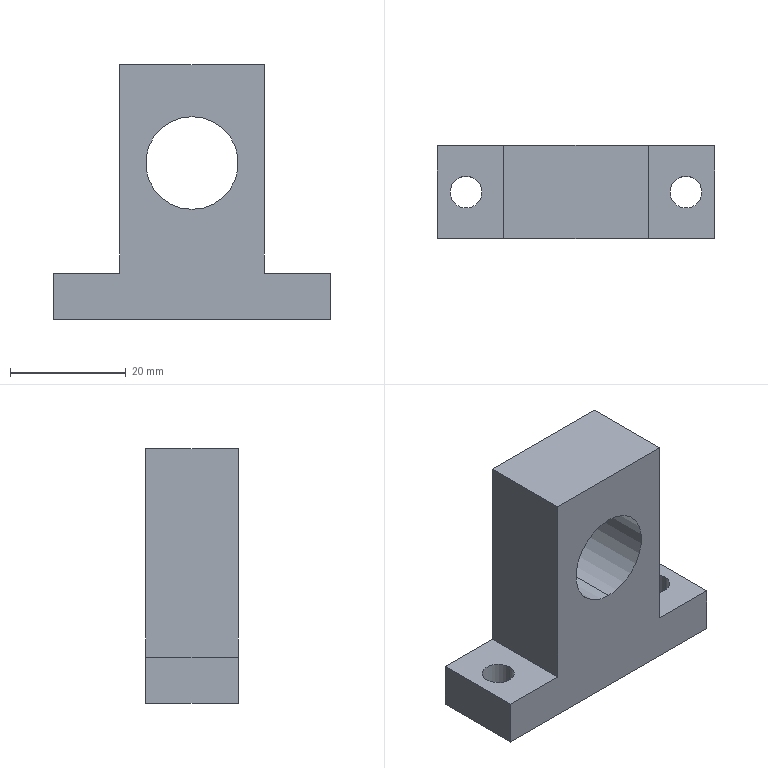Part | SolidWorks | features BaseBody 1 | 1 solid | 16 faces | box 48 x 16 x 44 mm | volume 16947 mm3 | plane 10 | cylinder 6 | commonest cylinder face diameters 5.5 x4 16 x2
STEP:
#1=CARTESIAN_POINT('',(0.,8.,19.));
#2=VERTEX_POINT('',#1);
#3=CARTESIAN_POINT('',(0.,8.,35.));
#4=VERTEX_POINT('',#3);
#5=CARTESIAN_POINT('',(0.,8.,27.));
#6=DIRECTION('',(0.,1.,0.));
#7=DIRECTION('',(0.,0.,-1.));
#8=AXIS2_PLACEMENT_3D('',#5,#6,#7);
#9=CIRCLE('',#8,8.);
#10=EDGE_CURVE('',#2,#4,#9,.T.);
#11=ORIENTED_EDGE('',*,*,#10,.T.);
#12=CARTESIAN_POINT('',(0.,-8.,35.));
#13=VERTEX_POINT('',#12);
#14=CARTESIAN_POINT('',(0.,8.,35.));
#15=DIRECTION('',(0.,-1.,0.));
#16=VECTOR('',#15,1000.);
#17=LINE('',#14,#16);
#18=EDGE_CURVE('',#4,#13,#17,.T.);
#19=ORIENTED_EDGE('',*,*,#18,.T.);
#20=CARTESIAN_POINT('',(0.,-8.,19.));
#21=VERTEX_POINT('',#20);
#22=CARTESIAN_POINT('',(0.,-8.,27.));
#23=DIRECTION('',(0.,1.,0.));
#24=DIRECTION('',(0.,0.,-1.));
#25=AXIS2_PLACEMENT_3D('',#22,#23,#24);
#26=CIRCLE('',#25,8.);
#27=EDGE_CURVE('',#21,#13,#26,.T.);
#28=ORIENTED_EDGE('',*,*,#27,.F.);
#29=CARTESIAN_POINT('',(0.,8.,19.));
#30=DIRECTION('',(0.,-1.,0.));
#31=VECTOR('',#30,1000.);
#32=LINE('',#29,#31);
#33=EDGE_CURVE('',#2,#21,#32,.T.);
#34=ORIENTED_EDGE('',*,*,#33,.F.);
#35=EDGE_LOOP('',(#11,#19,#28,#34));
#36=FACE_OUTER_BOUND('',#35,.T.);
#37=CARTESIAN_POINT('',(0.,8.,27.));
#38=DIRECTION('',(0.,-1.,0.));
#39=DIRECTION('',(0.,0.,-1.));
#40=AXIS2_PLACEMENT_3D('',#37,#38,#39);
#41=CYLINDRICAL_SURFACE('',#40,8.);
#42=ADVANCED_FACE('',(#36),#41,.F.);
#43=CARTESIAN_POINT('',(16.25,0.,8.));
#44=VERTEX_POINT('',#43);
#45=CARTESIAN_POINT('',(21.75,0.,8.));
#46=VERTEX_POINT('',#45);
#47=CARTESIAN_POINT('',(19.,0.,8.));
#48=DIRECTION('',(0.,0.,1.));
#49=DIRECTION('',(-1.,0.,0.));
#50=AXIS2_PLACEMENT_3D('',#47,#48,#49);
#51=CIRCLE('',#50,2.75);
#52=EDGE_CURVE('',#44,#46,#51,.T.);
#53=ORIENTED_EDGE('',*,*,#52,.T.);
#54=CARTESIAN_POINT('',(21.75,0.,0.));
#55=VERTEX_POINT('',#54);
#56=CARTESIAN_POINT('',(21.75,0.,8.));
#57=DIRECTION('',(0.,0.,-1.));
#58=VECTOR('',#57,1000.);
#59=LINE('',#56,#58);
#60=EDGE_CURVE('',#46,#55,#59,.T.);
#61=ORIENTED_EDGE('',*,*,#60,.T.);
#62=CARTESIAN_POINT('',(16.25,0.,0.));
#63=VERTEX_POINT('',#62);
#64=CARTESIAN_POINT('',(19.,0.,0.));
#65=DIRECTION('',(0.,0.,1.));
#66=DIRECTION('',(-1.,0.,0.));
#67=AXIS2_PLACEMENT_3D('',#64,#65,#66);
#68=CIRCLE('',#67,2.75);
#69=EDGE_CURVE('',#63,#55,#68,.T.);
#70=ORIENTED_EDGE('',*,*,#69,.F.);
#71=CARTESIAN_POINT('',(16.25,0.,8.));
#72=DIRECTION('',(0.,0.,-1.));
#73=VECTOR('',#72,1000.);
#74=LINE('',#71,#73);
#75=EDGE_CURVE('',#44,#63,#74,.T.);
#76=ORIENTED_EDGE('',*,*,#75,.F.);
#77=EDGE_LOOP('',(#53,#61,#70,#76));
#78=FACE_OUTER_BOUND('',#77,.T.);
#79=CARTESIAN_POINT('',(19.,0.,8.));
#80=DIRECTION('',(0.,0.,-1.));
#81=DIRECTION('',(-1.,0.,0.));
#82=AXIS2_PLACEMENT_3D('',#79,#80,#81);
#83=CYLINDRICAL_SURFACE('',#82,2.75);
#84=ADVANCED_FACE('',(#78),#83,.F.);
#85=CARTESIAN_POINT('',(-21.75,0.,8.));
#86=VERTEX_POINT('',#85);
#87=CARTESIAN_POINT('',(-16.25,0.,8.));
#88=VERTEX_POINT('',#87);
#89=CARTESIAN_POINT('',(-19.,0.,8.));
#90=DIRECTION('',(0.,0.,1.));
#91=DIRECTION('',(-1.,0.,0.));
#92=AXIS2_PLACEMENT_3D('',#89,#90,#91);
#93=CIRCLE('',#92,2.75);
#94=EDGE_CURVE('',#86,#88,#93,.T.);
#95=ORIENTED_EDGE('',*,*,#94,.T.);
#96=CARTESIAN_POINT('',(-16.25,0.,0.));
#97=VERTEX_POINT('',#96);
#98=CARTESIAN_POINT('',(-16.25,0.,8.));
#99=DIRECTION('',(0.,0.,-1.));
#100=VECTOR('',#99,1000.);
#101=LINE('',#98,#100);
#102=EDGE_CURVE('',#88,#97,#101,.T.);
#103=ORIENTED_EDGE('',*,*,#102,.T.);
#104=CARTESIAN_POINT('',(-21.75,0.,0.));
#105=VERTEX_POINT('',#104);
#106=CARTESIAN_POINT('',(-19.,0.,0.));
#107=DIRECTION('',(0.,0.,1.));
#108=DIRECTION('',(-1.,0.,0.));
#109=AXIS2_PLACEMENT_3D('',#106,#107,#108);
#110=CIRCLE('',#109,2.75);
#111=EDGE_CURVE('',#105,#97,#110,.T.);
#112=ORIENTED_EDGE('',*,*,#111,.F.);
#113=CARTESIAN_POINT('',(-21.75,0.,8.));
#114=DIRECTION('',(0.,0.,-1.));
#115=VECTOR('',#114,1000.);
#116=LINE('',#113,#115);
#117=EDGE_CURVE('',#86,#105,#116,.T.);
#118=ORIENTED_EDGE('',*,*,#117,.F.);
#119=EDGE_LOOP('',(#95,#103,#112,#118));
#120=FACE_OUTER_BOUND('',#119,.T.);
#121=CARTESIAN_POINT('',(-19.,0.,8.));
#122=DIRECTION('',(0.,0.,-1.));
#123=DIRECTION('',(-1.,0.,0.));
#124=AXIS2_PLACEMENT_3D('',#121,#122,#123);
#125=CYLINDRICAL_SURFACE('',#124,2.75);
#126=ADVANCED_FACE('',(#120),#125,.F.);
#127=ORIENTED_EDGE('',*,*,#10,.F.);
#128=CARTESIAN_POINT('',(0.,8.,27.));
#129=DIRECTION('',(0.,1.,0.));
#130=DIRECTION('',(0.,0.,-1.));
#131=AXIS2_PLACEMENT_3D('',#128,#129,#130);
#132=CIRCLE('',#131,8.);
#133=EDGE_CURVE('',#4,#2,#132,.T.);
#134=ORIENTED_EDGE('',*,*,#133,.F.);
#135=EDGE_LOOP('',(#127,#134));
#136=FACE_BOUND('',#135,.T.);
#137=CARTESIAN_POINT('',(-24.,8.,8.));
#138=VERTEX_POINT('',#137);
#139=CARTESIAN_POINT('',(-24.,8.,0.));
#140=VERTEX_POINT('',#139);
#141=CARTESIAN_POINT('',(-24.,8.,8.));
#142=DIRECTION('',(0.,0.,-1.));
#143=VECTOR('',#142,1000.);
#144=LINE('',#141,#143);
#145=EDGE_CURVE('',#138,#140,#144,.T.);
#146=ORIENTED_EDGE('',*,*,#145,.F.);
#147=CARTESIAN_POINT('',(-12.5,8.,8.));
#148=VERTEX_POINT('',#147);
#149=CARTESIAN_POINT('',(-24.,8.,8.));
#150=DIRECTION('',(-1.,0.,0.));
#151=VECTOR('',#150,1000.);
#152=LINE('',#149,#151);
#153=EDGE_CURVE('',#148,#138,#152,.T.);
#154=ORIENTED_EDGE('',*,*,#153,.F.);
#155=CARTESIAN_POINT('',(-12.5,8.,44.));
#156=VERTEX_POINT('',#155);
#157=CARTESIAN_POINT('',(-12.5,8.,8.));
#158=DIRECTION('',(0.,0.,-1.));
#159=VECTOR('',#158,1000.);
#160=LINE('',#157,#159);
#161=EDGE_CURVE('',#156,#148,#160,.T.);
#162=ORIENTED_EDGE('',*,*,#161,.F.);
#163=CARTESIAN_POINT('',(12.5,8.,44.));
#164=VERTEX_POINT('',#163);
#165=CARTESIAN_POINT('',(-24.,8.,44.));
#166=DIRECTION('',(-1.,0.,0.));
#167=VECTOR('',#166,1000.);
#168=LINE('',#165,#167);
#169=EDGE_CURVE('',#164,#156,#168,.T.);
#170=ORIENTED_EDGE('',*,*,#169,.F.);
#171=CARTESIAN_POINT('',(12.5,8.,8.));
#172=VERTEX_POINT('',#171);
#173=CARTESIAN_POINT('',(12.5,8.,8.));
#174=DIRECTION('',(0.,0.,1.));
#175=VECTOR('',#174,1000.);
#176=LINE('',#173,#175);
#177=EDGE_CURVE('',#172,#164,#176,.T.);
#178=ORIENTED_EDGE('',*,*,#177,.F.);
#179=CARTESIAN_POINT('',(24.,8.,8.));
#180=VERTEX_POINT('',#179);
#181=CARTESIAN_POINT('',(-24.,8.,8.));
#182=DIRECTION('',(-1.,0.,0.));
#183=VECTOR('',#182,1000.);
#184=LINE('',#181,#183);
#185=EDGE_CURVE('',#180,#172,#184,.T.);
#186=ORIENTED_EDGE('',*,*,#185,.F.);
#187=CARTESIAN_POINT('',(24.,8.,0.));
#188=VERTEX_POINT('',#187);
#189=CARTESIAN_POINT('',(24.,8.,8.));
#190=DIRECTION('',(0.,0.,1.));
#191=VECTOR('',#190,1000.);
#192=LINE('',#189,#191);
#193=EDGE_CURVE('',#188,#180,#192,.T.);
#194=ORIENTED_EDGE('',*,*,#193,.F.);
#195=CARTESIAN_POINT('',(-24.,8.,0.));
#196=DIRECTION('',(1.,0.,0.));
#197=VECTOR('',#196,1000.);
#198=LINE('',#195,#197);
#199=EDGE_CURVE('',#140,#188,#198,.T.);
#200=ORIENTED_EDGE('',*,*,#199,.F.);
#201=EDGE_LOOP('',(#146,#154,#162,#170,#178,#186,#194,#200));
#202=FACE_OUTER_BOUND('',#201,.T.);
#203=CARTESIAN_POINT('',(-24.,8.,8.));
#204=DIRECTION('',(0.,-1.,0.));
#205=DIRECTION('',(0.,0.,-1.));
#206=AXIS2_PLACEMENT_3D('',#203,#204,#205);
#207=PLANE('',#206);
#208=ADVANCED_FACE('',(#136,#202),#207,.F.);
#209=ORIENTED_EDGE('',*,*,#18,.F.);
#210=ORIENTED_EDGE('',*,*,#133,.T.);
#211=ORIENTED_EDGE('',*,*,#33,.T.);
#212=CARTESIAN_POINT('',(0.,-8.,27.));
#213=DIRECTION('',(0.,1.,0.));
#214=DIRECTION('',(0.,0.,-1.));
#215=AXIS2_PLACEMENT_3D('',#212,#213,#214);
#216=CIRCLE('',#215,8.);
#217=EDGE_CURVE('',#13,#21,#216,.T.);
#218=ORIENTED_EDGE('',*,*,#217,.F.);
#219=EDGE_LOOP('',(#209,#210,#211,#218));
#220=FACE_OUTER_BOUND('',#219,.T.);
#221=CARTESIAN_POINT('',(0.,8.,27.));
#222=DIRECTION('',(0.,-1.,0.));
#223=DIRECTION('',(0.,0.,-1.));
#224=AXIS2_PLACEMENT_3D('',#221,#222,#223);
#225=CYLINDRICAL_SURFACE('',#224,8.);
#226=ADVANCED_FACE('',(#220),#225,.F.);
#227=ORIENTED_EDGE('',*,*,#69,.T.);
#228=CARTESIAN_POINT('',(19.,0.,0.));
#229=DIRECTION('',(0.,0.,1.));
#230=DIRECTION('',(-1.,0.,0.));
#231=AXIS2_PLACEMENT_3D('',#228,#229,#230);
#232=CIRCLE('',#231,2.75);
#233=EDGE_CURVE('',#55,#63,#232,.T.);
#234=ORIENTED_EDGE('',*,*,#233,.T.);
#235=EDGE_LOOP('',(#227,#234));
#236=FACE_BOUND('',#235,.T.);
#237=CARTESIAN_POINT('',(-24.,-8.,0.));
#238=VERTEX_POINT('',#237);
#239=CARTESIAN_POINT('',(-24.,0.,0.));
#240=DIRECTION('',(0.,1.,0.));
#241=VECTOR('',#240,1000.);
#242=LINE('',#239,#241);
#243=EDGE_CURVE('',#238,#140,#242,.T.);
#244=ORIENTED_EDGE('',*,*,#243,.T.);
#245=ORIENTED_EDGE('',*,*,#199,.T.);
#246=CARTESIAN_POINT('',(24.,-8.,0.));
#247=VERTEX_POINT('',#246);
#248=CARTESIAN_POINT('',(24.,0.,0.));
#249=DIRECTION('',(0.,-1.,0.));
#250=VECTOR('',#249,1000.);
#251=LINE('',#248,#250);
#252=EDGE_CURVE('',#188,#247,#251,.T.);
#253=ORIENTED_EDGE('',*,*,#252,.T.);
#254=CARTESIAN_POINT('',(0.,-8.,0.));
#255=DIRECTION('',(-1.,0.,0.));
#256=VECTOR('',#255,1000.);
#257=LINE('',#254,#256);
#258=EDGE_CURVE('',#247,#238,#257,.T.);
#259=ORIENTED_EDGE('',*,*,#258,.T.);
#260=EDGE_LOOP('',(#244,#245,#253,#259));
#261=FACE_OUTER_BOUND('',#260,.T.);
#262=ORIENTED_EDGE('',*,*,#111,.T.);
#263=CARTESIAN_POINT('',(-19.,0.,0.));
#264=DIRECTION('',(0.,0.,1.));
#265=DIRECTION('',(-1.,0.,0.));
#266=AXIS2_PLACEMENT_3D('',#263,#264,#265);
#267=CIRCLE('',#266,2.75);
#268=EDGE_CURVE('',#97,#105,#267,.T.);
#269=ORIENTED_EDGE('',*,*,#268,.T.);
#270=EDGE_LOOP('',(#262,#269));
#271=FACE_BOUND('',#270,.T.);
#272=CARTESIAN_POINT('',(0.,0.,0.));
#273=DIRECTION('',(0.,0.,-1.));
#274=DIRECTION('',(-1.,0.,0.));
#275=AXIS2_PLACEMENT_3D('',#272,#273,#274);
#276=PLANE('',#275);
#277=ADVANCED_FACE('',(#236,#261,#271),#276,.T.);
#278=CARTESIAN_POINT('',(-24.,-8.,8.));
#279=VERTEX_POINT('',#278);
#280=CARTESIAN_POINT('',(-24.,-8.,8.));
#281=DIRECTION('',(0.,0.,-1.));
#282=VECTOR('',#281,1000.);
#283=LINE('',#280,#282);
#284=EDGE_CURVE('',#279,#238,#283,.T.);
#285=ORIENTED_EDGE('',*,*,#284,.F.);
#286=CARTESIAN_POINT('',(-24.,-8.,8.));
#287=DIRECTION('',(0.,-1.,0.));
#288=VECTOR('',#287,1000.);
#289=LINE('',#286,#288);
#290=EDGE_CURVE('',#138,#279,#289,.T.);
#291=ORIENTED_EDGE('',*,*,#290,.F.);
#292=ORIENTED_EDGE('',*,*,#145,.T.);
#293=ORIENTED_EDGE('',*,*,#243,.F.);
#294=EDGE_LOOP('',(#285,#291,#292,#293));
#295=FACE_OUTER_BOUND('',#294,.T.);
#296=CARTESIAN_POINT('',(-24.,-8.,8.));
#297=DIRECTION('',(1.,0.,0.));
#298=DIRECTION('',(0.,0.,-1.));
#299=AXIS2_PLACEMENT_3D('',#296,#297,#298);
#300=PLANE('',#299);
#301=ADVANCED_FACE('',(#295),#300,.F.);
#302=ORIENTED_EDGE('',*,*,#153,.T.);
#303=ORIENTED_EDGE('',*,*,#290,.T.);
#304=CARTESIAN_POINT('',(-12.5,-8.,8.));
#305=VERTEX_POINT('',#304);
#306=CARTESIAN_POINT('',(0.,-8.,8.));
#307=DIRECTION('',(-1.,0.,0.));
#308=VECTOR('',#307,1000.);
#309=LINE('',#306,#308);
#310=EDGE_CURVE('',#305,#279,#309,.T.);
#311=ORIENTED_EDGE('',*,*,#310,.F.);
#312=CARTESIAN_POINT('',(-12.5,0.,8.));
#313=DIRECTION('',(0.,-1.,0.));
#314=VECTOR('',#313,1000.);
#315=LINE('',#312,#314);
#316=EDGE_CURVE('',#148,#305,#315,.T.);
#317=ORIENTED_EDGE('',*,*,#316,.F.);
#318=EDGE_LOOP('',(#302,#303,#311,#317));
#319=FACE_OUTER_BOUND('',#318,.T.);
#320=ORIENTED_EDGE('',*,*,#94,.F.);
#321=CARTESIAN_POINT('',(-19.,0.,8.));
#322=DIRECTION('',(0.,0.,1.));
#323=DIRECTION('',(-1.,0.,0.));
#324=AXIS2_PLACEMENT_3D('',#321,#322,#323);
#325=CIRCLE('',#324,2.75);
#326=EDGE_CURVE('',#88,#86,#325,.T.);
#327=ORIENTED_EDGE('',*,*,#326,.F.);
#328=EDGE_LOOP('',(#320,#327));
#329=FACE_BOUND('',#328,.T.);
#330=CARTESIAN_POINT('',(0.,0.,8.));
#331=DIRECTION('',(0.,0.,-1.));
#332=DIRECTION('',(-1.,0.,0.));
#333=AXIS2_PLACEMENT_3D('',#330,#331,#332);
#334=PLANE('',#333);
#335=ADVANCED_FACE('',(#319,#329),#334,.F.);
#336=ORIENTED_EDGE('',*,*,#161,.T.);
#337=ORIENTED_EDGE('',*,*,#316,.T.);
#338=CARTESIAN_POINT('',(-12.5,-8.,44.));
#339=VERTEX_POINT('',#338);
#340=CARTESIAN_POINT('',(-12.5,-8.,8.));
#341=DIRECTION('',(0.,0.,1.));
#342=VECTOR('',#341,1000.);
#343=LINE('',#340,#342);
#344=EDGE_CURVE('',#305,#339,#343,.T.);
#345=ORIENTED_EDGE('',*,*,#344,.T.);
#346=CARTESIAN_POINT('',(-12.5,8.,44.));
#347=DIRECTION('',(0.,1.,0.));
#348=VECTOR('',#347,1000.);
#349=LINE('',#346,#348);
#350=EDGE_CURVE('',#339,#156,#349,.T.);
#351=ORIENTED_EDGE('',*,*,#350,.T.);
#352=EDGE_LOOP('',(#336,#337,#345,#351));
#353=FACE_OUTER_BOUND('',#352,.T.);
#354=CARTESIAN_POINT('',(-12.5,8.,8.));
#355=DIRECTION('',(-1.,0.,0.));
#356=DIRECTION('',(0.,0.,1.));
#357=AXIS2_PLACEMENT_3D('',#354,#355,#356);
#358=PLANE('',#357);
#359=ADVANCED_FACE('',(#353),#358,.T.);
#360=ORIENTED_EDGE('',*,*,#169,.T.);
#361=ORIENTED_EDGE('',*,*,#350,.F.);
#362=CARTESIAN_POINT('',(12.5,-8.,44.));
#363=VERTEX_POINT('',#362);
#364=CARTESIAN_POINT('',(-12.5,-8.,44.));
#365=DIRECTION('',(1.,0.,0.));
#366=VECTOR('',#365,1000.);
#367=LINE('',#364,#366);
#368=EDGE_CURVE('',#339,#363,#367,.T.);
#369=ORIENTED_EDGE('',*,*,#368,.T.);
#370=CARTESIAN_POINT('',(12.5,8.,44.));
#371=DIRECTION('',(0.,1.,0.));
#372=VECTOR('',#371,1000.);
#373=LINE('',#370,#372);
#374=EDGE_CURVE('',#363,#164,#373,.T.);
#375=ORIENTED_EDGE('',*,*,#374,.T.);
#376=EDGE_LOOP('',(#360,#361,#369,#375));
#377=FACE_OUTER_BOUND('',#376,.T.);
#378=CARTESIAN_POINT('',(-12.5,8.,44.));
#379=DIRECTION('',(0.,0.,1.));
#380=DIRECTION('',(1.,0.,0.));
#381=AXIS2_PLACEMENT_3D('',#378,#379,#380);
#382=PLANE('',#381);
#383=ADVANCED_FACE('',(#377),#382,.T.);
#384=ORIENTED_EDGE('',*,*,#177,.T.);
#385=ORIENTED_EDGE('',*,*,#374,.F.);
#386=CARTESIAN_POINT('',(12.5,-8.,8.));
#387=VERTEX_POINT('',#386);
#388=CARTESIAN_POINT('',(12.5,-8.,44.));
#389=DIRECTION('',(0.,0.,-1.));
#390=VECTOR('',#389,1000.);
#391=LINE('',#388,#390);
#392=EDGE_CURVE('',#363,#387,#391,.T.);
#393=ORIENTED_EDGE('',*,*,#392,.T.);
#394=CARTESIAN_POINT('',(12.5,8.,8.));
#395=DIRECTION('',(0.,1.,0.));
#396=VECTOR('',#395,1000.);
#397=LINE('',#394,#396);
#398=EDGE_CURVE('',#387,#172,#397,.T.);
#399=ORIENTED_EDGE('',*,*,#398,.T.);
#400=EDGE_LOOP('',(#384,#385,#393,#399));
#401=FACE_OUTER_BOUND('',#400,.T.);
#402=CARTESIAN_POINT('',(12.5,8.,44.));
#403=DIRECTION('',(1.,0.,0.));
#404=DIRECTION('',(0.,0.,-1.));
#405=AXIS2_PLACEMENT_3D('',#402,#403,#404);
#406=PLANE('',#405);
#407=ADVANCED_FACE('',(#401),#406,.T.);
#408=ORIENTED_EDGE('',*,*,#52,.F.);
#409=CARTESIAN_POINT('',(19.,0.,8.));
#410=DIRECTION('',(0.,0.,1.));
#411=DIRECTION('',(-1.,0.,0.));
#412=AXIS2_PLACEMENT_3D('',#409,#410,#411);
#413=CIRCLE('',#412,2.75);
#414=EDGE_CURVE('',#46,#44,#413,.T.);
#415=ORIENTED_EDGE('',*,*,#414,.F.);
#416=EDGE_LOOP('',(#408,#415));
#417=FACE_BOUND('',#416,.T.);
#418=ORIENTED_EDGE('',*,*,#398,.F.);
#419=CARTESIAN_POINT('',(24.,-8.,8.));
#420=VERTEX_POINT('',#419);
#421=CARTESIAN_POINT('',(0.,-8.,8.));
#422=DIRECTION('',(-1.,0.,0.));
#423=VECTOR('',#422,1000.);
#424=LINE('',#421,#423);
#425=EDGE_CURVE('',#420,#387,#424,.T.);
#426=ORIENTED_EDGE('',*,*,#425,.F.);
#427=CARTESIAN_POINT('',(24.,0.,8.));
#428=DIRECTION('',(0.,-1.,0.));
#429=VECTOR('',#428,1000.);
#430=LINE('',#427,#429);
#431=EDGE_CURVE('',#180,#420,#430,.T.);
#432=ORIENTED_EDGE('',*,*,#431,.F.);
#433=ORIENTED_EDGE('',*,*,#185,.T.);
#434=EDGE_LOOP('',(#418,#426,#432,#433));
#435=FACE_OUTER_BOUND('',#434,.T.);
#436=CARTESIAN_POINT('',(0.,0.,8.));
#437=DIRECTION('',(0.,0.,-1.));
#438=DIRECTION('',(-1.,0.,0.));
#439=AXIS2_PLACEMENT_3D('',#436,#437,#438);
#440=PLANE('',#439);
#441=ADVANCED_FACE('',(#417,#435),#440,.F.);
#442=ORIENTED_EDGE('',*,*,#193,.T.);
#443=ORIENTED_EDGE('',*,*,#431,.T.);
#444=CARTESIAN_POINT('',(24.,-8.,8.));
#445=DIRECTION('',(0.,0.,1.));
#446=VECTOR('',#445,1000.);
#447=LINE('',#444,#446);
#448=EDGE_CURVE('',#247,#420,#447,.T.);
#449=ORIENTED_EDGE('',*,*,#448,.F.);
#450=ORIENTED_EDGE('',*,*,#252,.F.);
#451=EDGE_LOOP('',(#442,#443,#449,#450));
#452=FACE_OUTER_BOUND('',#451,.T.);
#453=CARTESIAN_POINT('',(24.,-8.,8.));
#454=DIRECTION('',(-1.,0.,0.));
#455=DIRECTION('',(0.,0.,1.));
#456=AXIS2_PLACEMENT_3D('',#453,#454,#455);
#457=PLANE('',#456);
#458=ADVANCED_FACE('',(#452),#457,.F.);
#459=ORIENTED_EDGE('',*,*,#27,.T.);
#460=ORIENTED_EDGE('',*,*,#217,.T.);
#461=EDGE_LOOP('',(#459,#460));
#462=FACE_BOUND('',#461,.T.);
#463=ORIENTED_EDGE('',*,*,#448,.T.);
#464=ORIENTED_EDGE('',*,*,#425,.T.);
#465=ORIENTED_EDGE('',*,*,#392,.F.);
#466=ORIENTED_EDGE('',*,*,#368,.F.);
#467=ORIENTED_EDGE('',*,*,#344,.F.);
#468=ORIENTED_EDGE('',*,*,#310,.T.);
#469=ORIENTED_EDGE('',*,*,#284,.T.);
#470=ORIENTED_EDGE('',*,*,#258,.F.);
#471=EDGE_LOOP('',(#463,#464,#465,#466,#467,#468,#469,#470));
#472=FACE_OUTER_BOUND('',#471,.T.);
#473=CARTESIAN_POINT('',(-24.,-8.,8.));
#474=DIRECTION('',(0.,1.,0.));
#475=DIRECTION('',(0.,0.,1.));
#476=AXIS2_PLACEMENT_3D('',#473,#474,#475);
#477=PLANE('',#476);
#478=ADVANCED_FACE('',(#462,#472),#477,.F.);
#479=ORIENTED_EDGE('',*,*,#60,.F.);
#480=ORIENTED_EDGE('',*,*,#414,.T.);
#481=ORIENTED_EDGE('',*,*,#75,.T.);
#482=ORIENTED_EDGE('',*,*,#233,.F.);
#483=EDGE_LOOP('',(#479,#480,#481,#482));
#484=FACE_OUTER_BOUND('',#483,.T.);
#485=CARTESIAN_POINT('',(19.,0.,8.));
#486=DIRECTION('',(0.,0.,-1.));
#487=DIRECTION('',(-1.,0.,0.));
#488=AXIS2_PLACEMENT_3D('',#485,#486,#487);
#489=CYLINDRICAL_SURFACE('',#488,2.75);
#490=ADVANCED_FACE('',(#484),#489,.F.);
#491=ORIENTED_EDGE('',*,*,#102,.F.);
#492=ORIENTED_EDGE('',*,*,#326,.T.);
#493=ORIENTED_EDGE('',*,*,#117,.T.);
#494=ORIENTED_EDGE('',*,*,#268,.F.);
#495=EDGE_LOOP('',(#491,#492,#493,#494));
#496=FACE_OUTER_BOUND('',#495,.T.);
#497=CARTESIAN_POINT('',(-19.,0.,8.));
#498=DIRECTION('',(0.,0.,-1.));
#499=DIRECTION('',(-1.,0.,0.));
#500=AXIS2_PLACEMENT_3D('',#497,#498,#499);
#501=CYLINDRICAL_SURFACE('',#500,2.75);
#502=ADVANCED_FACE('',(#496),#501,.F.);
#503=CLOSED_SHELL('',(#42,#84,#126,#208,#226,#277,#301,#335,#359,#383,#407,#441,#458,#478,#490,#502));
#504=MANIFOLD_SOLID_BREP('',#503);
#505=CARTESIAN_POINT('',(0.,0.,0.));
#506=DIRECTION('',(0.,0.,1.));
#507=DIRECTION('',(1.,0.,0.));
#508=AXIS2_PLACEMENT_3D('',#505,#506,#507);
#509=(LENGTH_UNIT()NAMED_UNIT(*)SI_UNIT(.MILLI.,.METRE.));
#510=UNCERTAINTY_MEASURE_WITH_UNIT(LENGTH_MEASURE(0.00001),#509,'','');
#511=(NAMED_UNIT(*)PLANE_ANGLE_UNIT()SI_UNIT($,.RADIAN.));
#512=(NAMED_UNIT(*)SI_UNIT($,.STERADIAN.)SOLID_ANGLE_UNIT());
#513=(GEOMETRIC_REPRESENTATION_CONTEXT(3)GLOBAL_UNCERTAINTY_ASSIGNED_CONTEXT((#510))GLOBAL_UNIT_ASSIGNED_CONTEXT((#509,#511,#512))REPRESENTATION_CONTEXT('',''));
#514=ADVANCED_BREP_SHAPE_REPRESENTATION('',(#504,#508),#513);